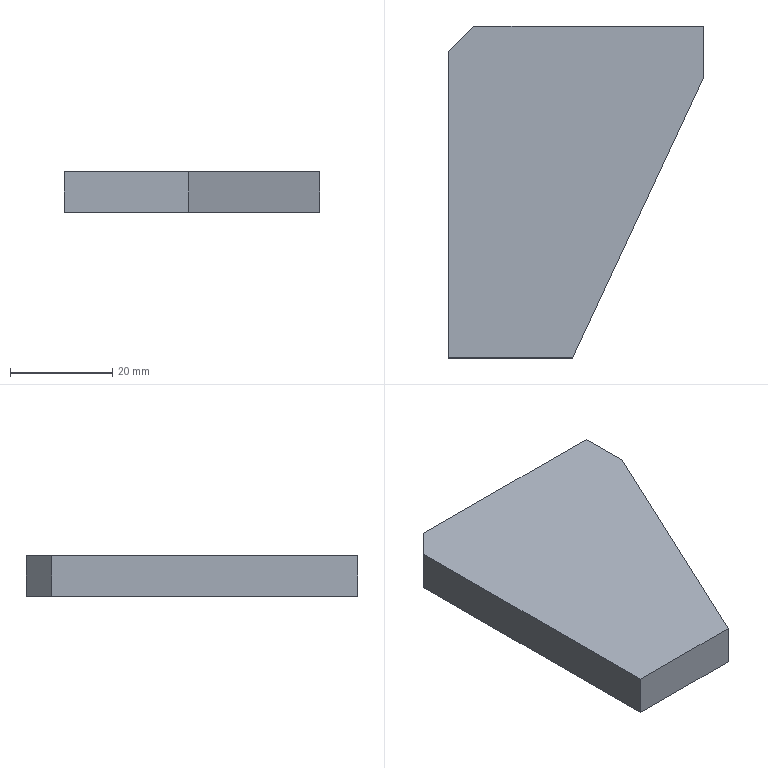Part | SolidWorks | features Chamfer 1, Extrusion 1 | 1 solid | 8 faces | box 50 x 65 x 8 mm | volume 20258 mm3 | plane 8
STEP:
#1=CARTESIAN_POINT('',(50.,55.,0.));
#2=VERTEX_POINT('',#1);
#3=CARTESIAN_POINT('',(50.,65.,0.));
#4=VERTEX_POINT('',#3);
#5=CARTESIAN_POINT('',(50.,65.,0.));
#6=DIRECTION('',(0.,1.,0.));
#7=VECTOR('',#6,1000.);
#8=LINE('',#5,#7);
#9=EDGE_CURVE('',#2,#4,#8,.T.);
#10=ORIENTED_EDGE('',*,*,#9,.T.);
#11=CARTESIAN_POINT('',(50.,65.,8.));
#12=VERTEX_POINT('',#11);
#13=CARTESIAN_POINT('',(50.,65.,8.));
#14=DIRECTION('',(0.,0.,-1.));
#15=VECTOR('',#14,1000.);
#16=LINE('',#13,#15);
#17=EDGE_CURVE('',#12,#4,#16,.T.);
#18=ORIENTED_EDGE('',*,*,#17,.F.);
#19=CARTESIAN_POINT('',(50.,55.,8.));
#20=VERTEX_POINT('',#19);
#21=CARTESIAN_POINT('',(50.,65.,8.));
#22=DIRECTION('',(0.,1.,0.));
#23=VECTOR('',#22,1000.);
#24=LINE('',#21,#23);
#25=EDGE_CURVE('',#20,#12,#24,.T.);
#26=ORIENTED_EDGE('',*,*,#25,.F.);
#27=CARTESIAN_POINT('',(50.,55.,8.));
#28=DIRECTION('',(0.,0.,-1.));
#29=VECTOR('',#28,1000.);
#30=LINE('',#27,#29);
#31=EDGE_CURVE('',#20,#2,#30,.T.);
#32=ORIENTED_EDGE('',*,*,#31,.T.);
#33=EDGE_LOOP('',(#10,#18,#26,#32));
#34=FACE_OUTER_BOUND('',#33,.T.);
#35=CARTESIAN_POINT('',(50.,65.,8.));
#36=DIRECTION('',(-1.,0.,0.));
#37=DIRECTION('',(0.,0.,1.));
#38=AXIS2_PLACEMENT_3D('',#35,#36,#37);
#39=PLANE('',#38);
#40=ADVANCED_FACE('',(#34),#39,.F.);
#41=CARTESIAN_POINT('',(5.,65.,0.));
#42=VERTEX_POINT('',#41);
#43=CARTESIAN_POINT('',(50.,65.,0.));
#44=DIRECTION('',(-1.,0.,0.));
#45=VECTOR('',#44,1000.);
#46=LINE('',#43,#45);
#47=EDGE_CURVE('',#4,#42,#46,.T.);
#48=ORIENTED_EDGE('',*,*,#47,.T.);
#49=CARTESIAN_POINT('',(5.,65.,8.));
#50=VERTEX_POINT('',#49);
#51=CARTESIAN_POINT('',(5.,65.,8.));
#52=DIRECTION('',(0.,0.,1.));
#53=VECTOR('',#52,1000.);
#54=LINE('',#51,#53);
#55=EDGE_CURVE('',#42,#50,#54,.T.);
#56=ORIENTED_EDGE('',*,*,#55,.T.);
#57=CARTESIAN_POINT('',(50.,65.,8.));
#58=DIRECTION('',(-1.,0.,0.));
#59=VECTOR('',#58,1000.);
#60=LINE('',#57,#59);
#61=EDGE_CURVE('',#12,#50,#60,.T.);
#62=ORIENTED_EDGE('',*,*,#61,.F.);
#63=ORIENTED_EDGE('',*,*,#17,.T.);
#64=EDGE_LOOP('',(#48,#56,#62,#63));
#65=FACE_OUTER_BOUND('',#64,.T.);
#66=CARTESIAN_POINT('',(50.,65.,8.));
#67=DIRECTION('',(0.,-1.,0.));
#68=DIRECTION('',(1.,0.,0.));
#69=AXIS2_PLACEMENT_3D('',#66,#67,#68);
#70=PLANE('',#69);
#71=ADVANCED_FACE('',(#65),#70,.F.);
#72=CARTESIAN_POINT('',(0.,60.,8.));
#73=VERTEX_POINT('',#72);
#74=CARTESIAN_POINT('',(0.,0.,8.));
#75=VERTEX_POINT('',#74);
#76=CARTESIAN_POINT('',(0.,65.,8.));
#77=DIRECTION('',(0.,-1.,0.));
#78=VECTOR('',#77,1000.);
#79=LINE('',#76,#78);
#80=EDGE_CURVE('',#73,#75,#79,.T.);
#81=ORIENTED_EDGE('',*,*,#80,.F.);
#82=CARTESIAN_POINT('',(0.,60.,0.));
#83=VERTEX_POINT('',#82);
#84=CARTESIAN_POINT('',(0.,60.,8.));
#85=DIRECTION('',(0.,0.,-1.));
#86=VECTOR('',#85,1000.);
#87=LINE('',#84,#86);
#88=EDGE_CURVE('',#73,#83,#87,.T.);
#89=ORIENTED_EDGE('',*,*,#88,.T.);
#90=CARTESIAN_POINT('',(0.,0.,0.));
#91=VERTEX_POINT('',#90);
#92=CARTESIAN_POINT('',(0.,65.,0.));
#93=DIRECTION('',(0.,-1.,0.));
#94=VECTOR('',#93,1000.);
#95=LINE('',#92,#94);
#96=EDGE_CURVE('',#83,#91,#95,.T.);
#97=ORIENTED_EDGE('',*,*,#96,.T.);
#98=CARTESIAN_POINT('',(0.,0.,8.));
#99=DIRECTION('',(0.,0.,-1.));
#100=VECTOR('',#99,1000.);
#101=LINE('',#98,#100);
#102=EDGE_CURVE('',#75,#91,#101,.T.);
#103=ORIENTED_EDGE('',*,*,#102,.F.);
#104=EDGE_LOOP('',(#81,#89,#97,#103));
#105=FACE_OUTER_BOUND('',#104,.T.);
#106=CARTESIAN_POINT('',(0.,65.,8.));
#107=DIRECTION('',(1.,0.,0.));
#108=DIRECTION('',(0.,1.,0.));
#109=AXIS2_PLACEMENT_3D('',#106,#107,#108);
#110=PLANE('',#109);
#111=ADVANCED_FACE('',(#105),#110,.F.);
#112=CARTESIAN_POINT('',(24.353,0.,0.));
#113=VERTEX_POINT('',#112);
#114=CARTESIAN_POINT('',(0.,0.,0.));
#115=DIRECTION('',(1.,0.,0.));
#116=VECTOR('',#115,1000.);
#117=LINE('',#114,#116);
#118=EDGE_CURVE('',#91,#113,#117,.T.);
#119=ORIENTED_EDGE('',*,*,#118,.T.);
#120=CARTESIAN_POINT('',(24.353,0.,8.));
#121=VERTEX_POINT('',#120);
#122=CARTESIAN_POINT('',(24.353,0.,8.));
#123=DIRECTION('',(0.,0.,-1.));
#124=VECTOR('',#123,1000.);
#125=LINE('',#122,#124);
#126=EDGE_CURVE('',#121,#113,#125,.T.);
#127=ORIENTED_EDGE('',*,*,#126,.F.);
#128=CARTESIAN_POINT('',(0.,0.,8.));
#129=DIRECTION('',(1.,0.,0.));
#130=VECTOR('',#129,1000.);
#131=LINE('',#128,#130);
#132=EDGE_CURVE('',#75,#121,#131,.T.);
#133=ORIENTED_EDGE('',*,*,#132,.F.);
#134=ORIENTED_EDGE('',*,*,#102,.T.);
#135=EDGE_LOOP('',(#119,#127,#133,#134));
#136=FACE_OUTER_BOUND('',#135,.T.);
#137=CARTESIAN_POINT('',(0.,0.,8.));
#138=DIRECTION('',(0.,1.,0.));
#139=DIRECTION('',(0.,0.,1.));
#140=AXIS2_PLACEMENT_3D('',#137,#138,#139);
#141=PLANE('',#140);
#142=ADVANCED_FACE('',(#136),#141,.F.);
#143=CARTESIAN_POINT('',(50.,55.,0.));
#144=DIRECTION('',(0.4226,0.9063,0.));
#145=VECTOR('',#144,1000.);
#146=LINE('',#143,#145);
#147=EDGE_CURVE('',#113,#2,#146,.T.);
#148=ORIENTED_EDGE('',*,*,#147,.T.);
#149=ORIENTED_EDGE('',*,*,#31,.F.);
#150=CARTESIAN_POINT('',(50.,55.,8.));
#151=DIRECTION('',(0.4226,0.9063,0.));
#152=VECTOR('',#151,1000.);
#153=LINE('',#150,#152);
#154=EDGE_CURVE('',#121,#20,#153,.T.);
#155=ORIENTED_EDGE('',*,*,#154,.F.);
#156=ORIENTED_EDGE('',*,*,#126,.T.);
#157=EDGE_LOOP('',(#148,#149,#155,#156));
#158=FACE_OUTER_BOUND('',#157,.T.);
#159=CARTESIAN_POINT('',(50.,55.,8.));
#160=DIRECTION('',(-0.9063,0.4226,0.));
#161=DIRECTION('',(-0.4226,-0.9063,0.));
#162=AXIS2_PLACEMENT_3D('',#159,#160,#161);
#163=PLANE('',#162);
#164=ADVANCED_FACE('',(#158),#163,.F.);
#165=ORIENTED_EDGE('',*,*,#61,.T.);
#166=CARTESIAN_POINT('',(-30.,30.,8.));
#167=DIRECTION('',(-0.7071,-0.7071,0.));
#168=VECTOR('',#167,1000.);
#169=LINE('',#166,#168);
#170=EDGE_CURVE('',#50,#73,#169,.T.);
#171=ORIENTED_EDGE('',*,*,#170,.T.);
#172=ORIENTED_EDGE('',*,*,#80,.T.);
#173=ORIENTED_EDGE('',*,*,#132,.T.);
#174=ORIENTED_EDGE('',*,*,#154,.T.);
#175=ORIENTED_EDGE('',*,*,#25,.T.);
#176=EDGE_LOOP('',(#165,#171,#172,#173,#174,#175));
#177=FACE_OUTER_BOUND('',#176,.T.);
#178=CARTESIAN_POINT('',(0.,0.,8.));
#179=DIRECTION('',(0.,0.,1.));
#180=DIRECTION('',(1.,0.,0.));
#181=AXIS2_PLACEMENT_3D('',#178,#179,#180);
#182=PLANE('',#181);
#183=ADVANCED_FACE('',(#177),#182,.T.);
#184=ORIENTED_EDGE('',*,*,#96,.F.);
#185=CARTESIAN_POINT('',(0.,60.,0.));
#186=DIRECTION('',(0.7071,0.7071,0.));
#187=VECTOR('',#186,1000.);
#188=LINE('',#185,#187);
#189=EDGE_CURVE('',#83,#42,#188,.T.);
#190=ORIENTED_EDGE('',*,*,#189,.T.);
#191=ORIENTED_EDGE('',*,*,#47,.F.);
#192=ORIENTED_EDGE('',*,*,#9,.F.);
#193=ORIENTED_EDGE('',*,*,#147,.F.);
#194=ORIENTED_EDGE('',*,*,#118,.F.);
#195=EDGE_LOOP('',(#184,#190,#191,#192,#193,#194));
#196=FACE_OUTER_BOUND('',#195,.T.);
#197=CARTESIAN_POINT('',(0.,0.,0.));
#198=DIRECTION('',(0.,0.,1.));
#199=DIRECTION('',(1.,0.,0.));
#200=AXIS2_PLACEMENT_3D('',#197,#198,#199);
#201=PLANE('',#200);
#202=ADVANCED_FACE('',(#196),#201,.F.);
#203=ORIENTED_EDGE('',*,*,#170,.F.);
#204=ORIENTED_EDGE('',*,*,#55,.F.);
#205=ORIENTED_EDGE('',*,*,#189,.F.);
#206=ORIENTED_EDGE('',*,*,#88,.F.);
#207=EDGE_LOOP('',(#203,#204,#205,#206));
#208=FACE_OUTER_BOUND('',#207,.T.);
#209=CARTESIAN_POINT('',(0.,60.,8.));
#210=DIRECTION('',(0.7071,-0.7071,0.));
#211=DIRECTION('',(0.,0.,-1.));
#212=AXIS2_PLACEMENT_3D('',#209,#210,#211);
#213=PLANE('',#212);
#214=ADVANCED_FACE('',(#208),#213,.F.);
#215=CLOSED_SHELL('',(#40,#71,#111,#142,#164,#183,#202,#214));
#216=MANIFOLD_SOLID_BREP('',#215);
#217=CARTESIAN_POINT('',(0.,0.,0.));
#218=DIRECTION('',(0.,0.,1.));
#219=DIRECTION('',(1.,0.,0.));
#220=AXIS2_PLACEMENT_3D('',#217,#218,#219);
#221=(LENGTH_UNIT()NAMED_UNIT(*)SI_UNIT(.MILLI.,.METRE.));
#222=UNCERTAINTY_MEASURE_WITH_UNIT(LENGTH_MEASURE(0.00001),#221,'','');
#223=(NAMED_UNIT(*)PLANE_ANGLE_UNIT()SI_UNIT($,.RADIAN.));
#224=(NAMED_UNIT(*)SI_UNIT($,.STERADIAN.)SOLID_ANGLE_UNIT());
#225=(GEOMETRIC_REPRESENTATION_CONTEXT(3)GLOBAL_UNCERTAINTY_ASSIGNED_CONTEXT((#222))GLOBAL_UNIT_ASSIGNED_CONTEXT((#221,#223,#224))REPRESENTATION_CONTEXT('',''));
#226=ADVANCED_BREP_SHAPE_REPRESENTATION('',(#216,#220),#225);